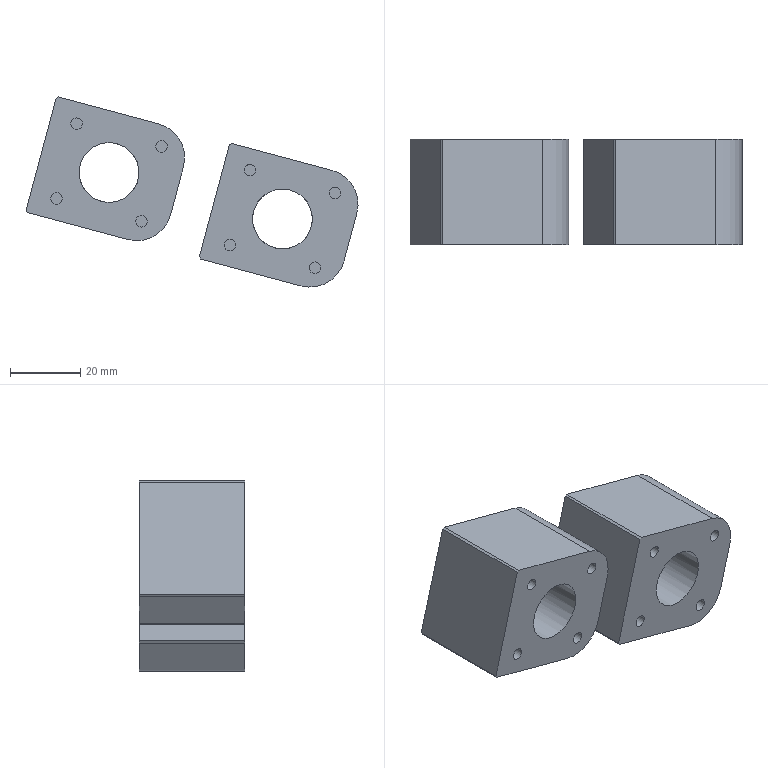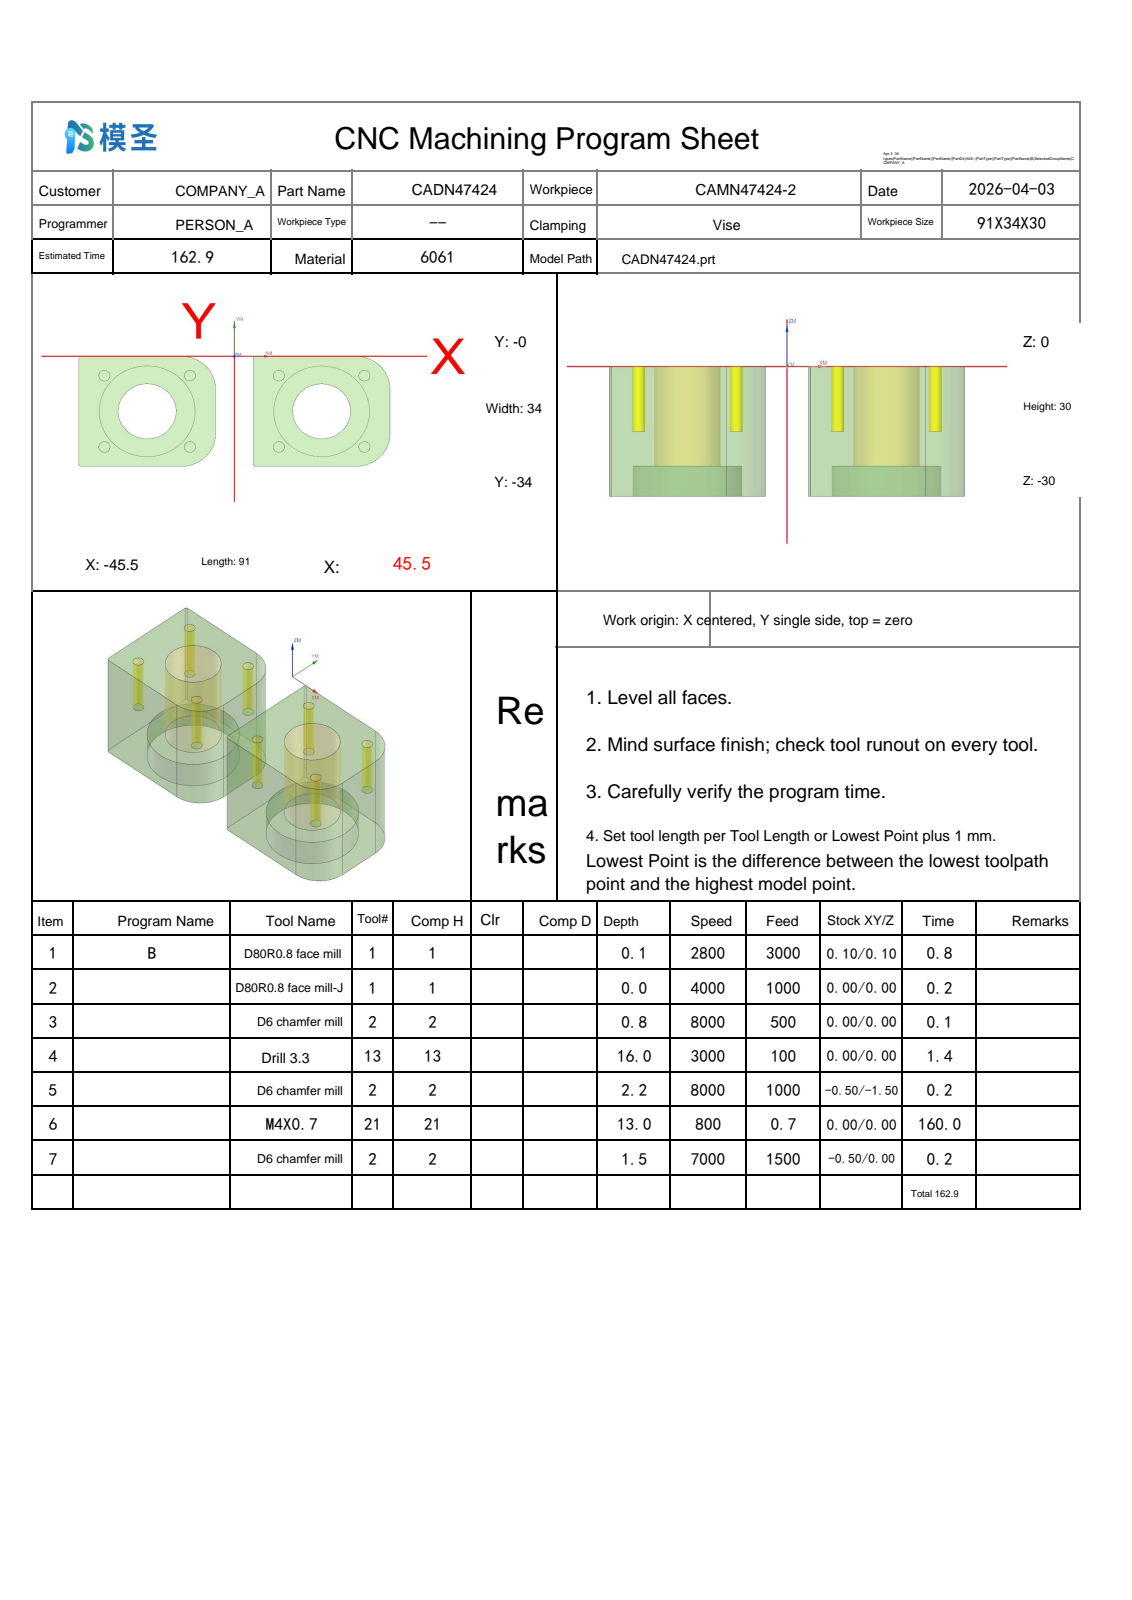NC program | NX | posted by the shop | part box 94.322 x 30 x 54.017 mm
Whole program:
%
O0001
(Machine time: 312.81 MIN)
(===Total Tool:4===)
(T1=D80R0.8 face mill D=80.  R=0.8  D-  H01 Z=0.    )
(T2=D6 chamfer mill   D=6.   R=0.   D-  H02 Z=-2.2  )
(T13=drill 3.3  D=3.3  DR_a=118 D-  H13 Z=-16.  )
(T21=M4X0.7 D=3.3  DR_a=180 D-  H21 Z=-13.  )
G80 G90 G17 G49 G40
G91 G28 Z0
M01
N1 T01 M06
(D80R0.8 face mill  D=80. R=0.8 H=01 ce=0.10 di=0.10)
G00 G90 G54 X97.597 Y-15.121 M03 S2800
G43 H01 Z20.
M08
Z6.011
G01 Z4.011 F3000.
X85.597 Y-15.341
X-85.597 Y-18.485
X-97.597 Y-18.706
Z6.011
G00 X97.597 Y-15.121
Z5.522
G01 Z3.522
X85.597 Y-15.341
X-85.597 Y-18.485
X-97.597 Y-18.706
Z5.522
G00 X97.597 Y-15.121
Z5.033
G01 Z3.033
X85.597 Y-15.341
X-85.597 Y-18.485
X-97.597 Y-18.706
Z5.033
G00 X97.597 Y-15.121
Z4.544
G01 Z2.544
X85.597 Y-15.341
X-85.597 Y-18.485
X-97.597 Y-18.706
Z4.544
G00 Z20.
X97.597 Y-15.121
Z4.056
G01 Z2.056
X85.597 Y-15.341
X-85.597 Y-18.485
X-97.597 Y-18.706
Z4.056
G00 Z20.
X97.597 Y-15.121
Z3.567
G01 Z1.567
X85.597 Y-15.341
X-85.597 Y-18.485
X-97.597 Y-18.706
Z3.567
G00 Z20.
X97.597 Y-15.121
Z3.078
G01 Z1.078
X85.597 Y-15.341
X-85.597 Y-18.485
X-97.597 Y-18.706
Z3.078
G00 Z20.
X97.597 Y-15.121
Z2.589
G01 Z.589
X85.597 Y-15.341
X-85.597 Y-18.485
X-97.597 Y-18.706
Z2.589
G00 Z20.
X97.597 Y-15.121
Z2.1
G01 Z.1
X85.597 Y-15.341
X-85.597 Y-18.485
X-97.597 Y-18.706
Z2.1
G00 Z20.
G91 G28 Z0.0
M05
M09
G91 G28 Z0.0
M01
N2 T01 M06
(D80R0.8 face mill-J  D=80. R=0.8 H=01 ce=0.00 di=0.00)
G00 G90 G54 X97.499 Y-15.125 M03 S4000
G43 H01 Z20.
M08
Z2.
G01 Z0.0 F1000.
X85.499 Y-15.345
X-85.499 Y-18.482
X-97.499 Y-18.702
Z2.
G00 Z20.
G91 G28 Z0.0
M05
M09
G91 G28 Z0.0
M01
N3 T02 M06
(D6 chamfer mill  D=6. R=0. H=02 ce=0.00 di=0.00)
G00 G90 G54 X-38. Y-6. M03 S8000
G43 H02 Z20.
M08
G98 G81 X-38. Y-6. Z-.8 R1. F500.
Y-28.
X-25.5 Y-17.
X-13. Y-6.
Y-28.
X13.
Y-6.
X25.5 Y-17.
X38. Y-28.
Y-6.
G80
G00 Z20.
G91 G28 Z0.0
M05
M09
G91 G28 Z0.0
M01
N4 T13 M06
(drill 3.3 D=3.3 DR_a=118 H=13)
G00 G90 G54 X38. Y-6. M03 S3000
G43 H13 Z20.
M08
G98 G83 X38. Y-6. Z-16. R1. F100. Q2.
Y-28.
X13.
Y-6.
X-13.
Y-28.
X-38.
Y-6.
G80
G00 Z20.
G91 G28 Z0.0
M05
M09
G91 G28 Z0.0
M01
N5 T02 M06
(D6 chamfer mill  D=6. R=0. H=02 ce=0.00 di=0.00)
G00 G90 G54 X38. Y-6. M03 S8000
G43 H02 Z20.
M08
G98 G81 X38. Y-6. Z-2.2 R3. F500.
Y-28.
X13.
Y-6.
X-13.
Y-28.
X-38.
Y-6.
G80
G00 Z20.
G00 G90 X-23.767 Y-11.877 M03 S8000
Z20.
Z-1.
G01 Z-1.5 F1000.
G03 X-26.665 Y-9.653 I-2.898 J-.776
X-27.441 Y-9.756 I0.0 J-3.
X-33. Y-17. I1.941 J-7.244
X-25.5 Y-24.5 I7.5 J0.0
X-18. Y-17. I0.0 J7.5
X-25.5 Y-9.5 I-7.5 J0.0
X-27.441 Y-9.756 I0.0 J-7.5
X-29.665 Y-12.653 I.776 J-2.898
X-29.562 Y-13.43 I3. J0.0
G01 Z-1.
G00 Z20.
X27.233 Y-11.877
Z-1.
G01 Z-1.5
G03 X24.335 Y-9.653 I-2.898 J-.776
X23.559 Y-9.756 I0.0 J-3.
X18. Y-17. I1.941 J-7.244
X25.5 Y-24.5 I7.5 J0.0
X33. Y-17. I0.0 J7.5
X25.5 Y-9.5 I-7.5 J0.0
X23.559 Y-9.756 I0.0 J-7.5
X21.335 Y-12.653 I.776 J-2.898
X21.438 Y-13.43 I3. J0.0
G01 Z-1.
G00 Z20.
G91 G28 Z0.0
M05
M09
G91 G28 Z0.0
M01
N6 T21 M06
(M4X0.7 D=3.3 DR_a=180 H=21)
G00 G90 G54 X38. Y-6. M03 S800
G43 H21 Z20.
M08
G95
G98 G84 X38. Y-6. Z-13. R1. F.7 Q4.
Y-28.
X13.
Y-6.
X-13.
Y-28.
X-38.
Y-6.
G80
G94
G00 Z20.
G91 G28 Z0.0
M05
M09
G91 G28 Z0.0
M01
N7 T02 M06
(D6 chamfer mill  D=6. R=0. H=02 ce=-0.50 di=0.00)
G00 G90 G54 X41.452 Y-.752 M03 S7000
G43 H02 Z20.
M08
Z2.5
G01 X41.666 Y-.887 Z2.408 F1500.
X42.232 Y-1.297 Z2.153
X42.771 Y-1.742 Z1.899
X43.28 Y-2.22 Z1.645
X43.758 Y-2.729 Z1.391
X44.203 Y-3.268 Z1.136
X44.613 Y-3.834 Z.882
X44.986 Y-4.424 Z.628
X45.32 Y-5.038 Z.373
X45.616 Y-5.671 Z.119
X45.87 Y-6.322 Z-.135
X46.082 Y-6.987 Z-.389
X46.252 Y-7.665 Z-.644
X46.379 Y-8.352 Z-.898
X46.462 Y-9.046 Z-1.152
X46.5 Y-9.743 Z-1.406
Y-10. Z-1.5
Y-24.
G02 X35.5 Y-35. I-11. J0.0
G01 X6.207
G02 X5.146 Y-34.561 I0.0 J1.5
G01 X4.939 Y-34.354
G02 X4.5 Y-33.293 I1.061 J1.061
G01 Y-.707
G02 X4.939 Y.354 I1.5 J0.0
G01 X5.146 Y.561
G02 X6.207 Y1. I1.061 J-1.061
G01 X35.5
G02 X46.5 Y-10. I0.0 J-11.
G01 Y-10.5
Z1.
G00 Z20.
X-9.548 Y-.752
Z2.5
G01 X-9.334 Y-.887 Z2.408
X-8.768 Y-1.297 Z2.153
X-8.229 Y-1.742 Z1.899
X-7.72 Y-2.22 Z1.645
X-7.242 Y-2.729 Z1.391
X-6.797 Y-3.268 Z1.136
X-6.387 Y-3.834 Z.882
X-6.014 Y-4.424 Z.628
X-5.68 Y-5.038 Z.373
X-5.384 Y-5.671 Z.119
X-5.13 Y-6.322 Z-.135
X-4.918 Y-6.987 Z-.389
X-4.748 Y-7.665 Z-.644
X-4.621 Y-8.352 Z-.898
X-4.538 Y-9.046 Z-1.152
X-4.5 Y-9.743 Z-1.406
Y-10. Z-1.5
Y-24.
G02 X-15.5 Y-35. I-11. J0.0
G01 X-44.793
G02 X-45.854 Y-34.561 I0.0 J1.5
G01 X-46.061 Y-34.354
G02 X-46.5 Y-33.293 I1.061 J1.061
G01 Y-.707
G02 X-46.061 Y.354 I1.5 J0.0
G01 X-45.854 Y.561
G02 X-44.793 Y1. I1.061 J-1.061
G01 X-15.5
G02 X-4.5 Y-10. I0.0 J-11.
G01 Y-10.5
Z1.
G00 Z20.
M05
M09
G91 G28 Z0.0
G91 G28 Y0.0
M30
%